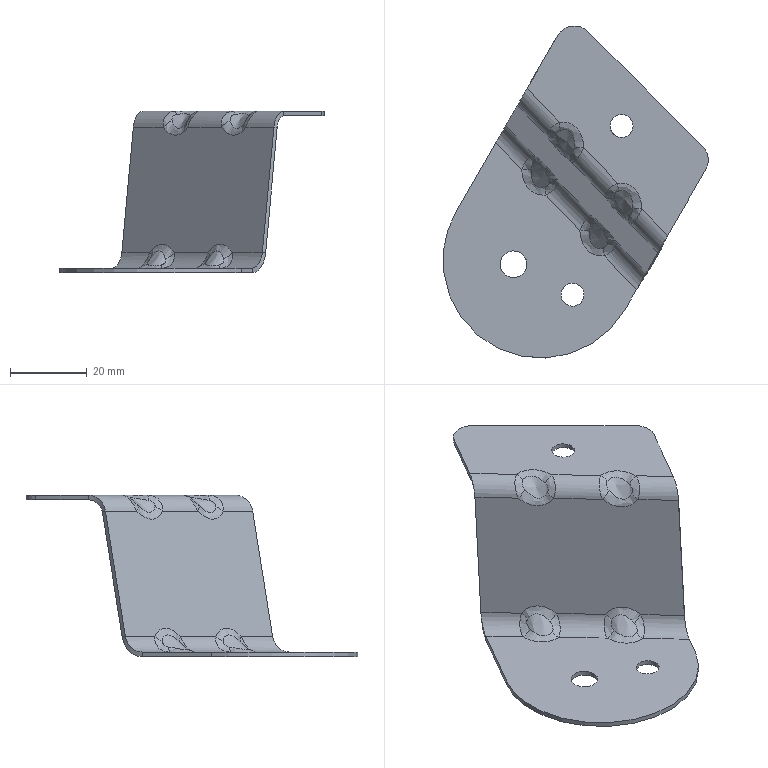Part | 1 solid | 78 faces | box 69.274 x 86.673 x 42.167 mm | volume 6319 mm3 | spline 49 | cylinder 21 | plane 8 | commonest cylinder face diameters 10 x8 6 x4 7.6 x3 12.4 x3 7 x2 51 x1